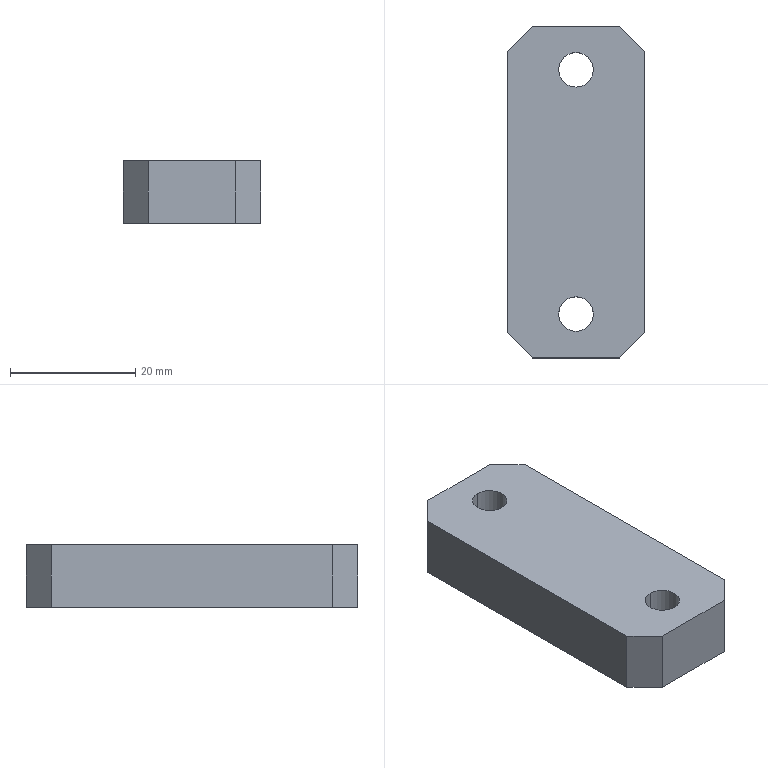Part | Creo | 1 solid | 110 faces | box 22 x 53 x 10 mm | volume 10297 mm3 | other 71 | plane 29 | cylinder 10 | commonest cylinder face diameters 5.5 x4 9.5 x4 2.89 x1 45.582 x1